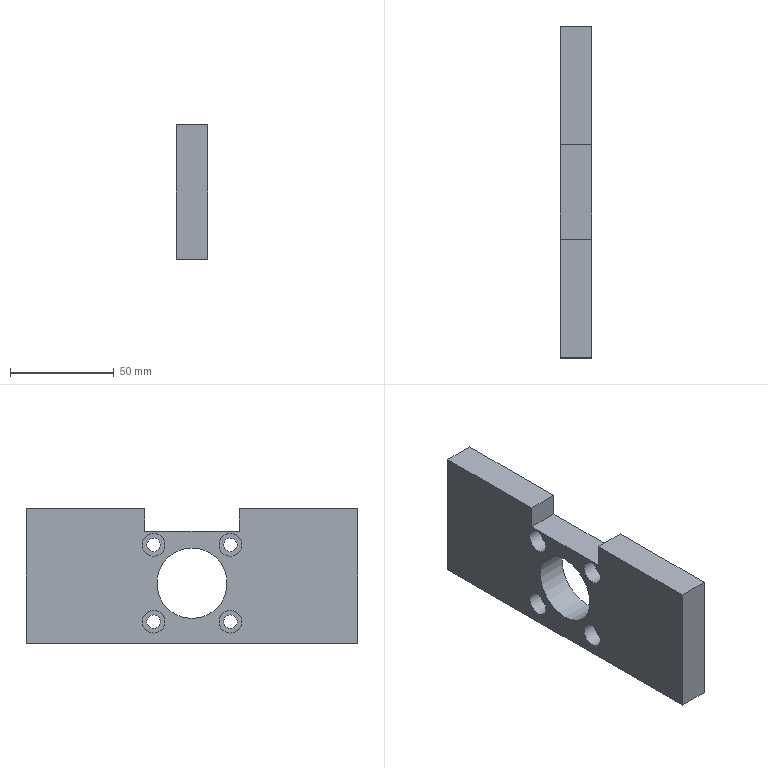Part | STEP file | Tube feed_id790_x_t | 1 solid | 23 faces | box 15 x 160 x 65 mm | volume 131151 mm3 | plane 14 | cylinder 9 | commonest cylinder face diameters 6.5 x4 11 x4 34 x1